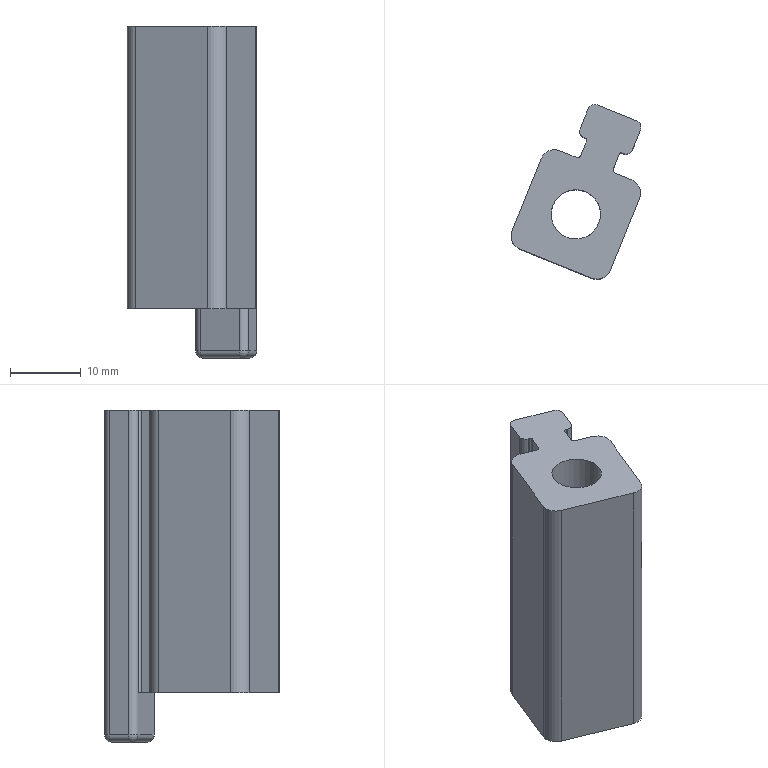Part | NX | features PS-13 2 | 1 solid | 37 faces | box 18.38 x 24.724 x 47 mm | volume 8910 mm3 | cylinder 18 | plane 15 | sphere 4 | commonest cylinder face diameters 2 x8 4 x4 0.6 x2 1 x2 7 x1 11 x1
STEP:
#1=CARTESIAN_POINT('',(2674.028,-826.139,860.716));
#2=VERTEX_POINT('',#1);
#3=CARTESIAN_POINT('',(2671.712,-825.199,860.716));
#4=VERTEX_POINT('',#3);
#5=CARTESIAN_POINT('',(89.829,221.566,860.716));
#6=DIRECTION('',(-0.9267,0.3757,0.));
#7=VECTOR('',#6,1000.);
#8=LINE('',#5,#7);
#9=EDGE_CURVE('',#2,#4,#8,.T.);
#10=ORIENTED_EDGE('',*,*,#9,.T.);
#11=CARTESIAN_POINT('',(2671.712,-825.199,900.716));
#12=VERTEX_POINT('',#11);
#13=CARTESIAN_POINT('',(2671.712,-825.199,900.716));
#14=DIRECTION('',(0.000000001,0.000000001,1.));
#15=VECTOR('',#14,1000.);
#16=LINE('',#13,#15);
#17=EDGE_CURVE('',#4,#12,#16,.T.);
#18=ORIENTED_EDGE('',*,*,#17,.T.);
#19=CARTESIAN_POINT('',(2674.028,-826.139,900.716));
#20=VERTEX_POINT('',#19);
#21=CARTESIAN_POINT('',(687.415,-20.712,900.716));
#22=DIRECTION('',(0.9267,-0.3757,0.));
#23=VECTOR('',#22,1000.);
#24=LINE('',#21,#23);
#25=EDGE_CURVE('',#20,#12,#24,.F.);
#26=ORIENTED_EDGE('',*,*,#25,.F.);
#27=CARTESIAN_POINT('',(2674.028,-826.139,880.716));
#28=DIRECTION('',(-0.000000001,-0.000000001,-1.));
#29=VECTOR('',#28,1000.);
#30=LINE('',#27,#29);
#31=EDGE_CURVE('',#20,#2,#30,.T.);
#32=ORIENTED_EDGE('',*,*,#31,.T.);
#33=EDGE_LOOP('',(#10,#18,#26,#32));
#34=FACE_BOUND('',#33,.T.);
#35=CARTESIAN_POINT('',(2672.638,-825.575,880.716));
#36=DIRECTION('',(0.3757,0.9267,-0.000000001));
#37=DIRECTION('',(-0.9267,0.3757,0.));
#38=AXIS2_PLACEMENT_3D('',#35,#36,#37);
#39=PLANE('',#38);
#40=ADVANCED_FACE('',(#34),#39,.T.);
#41=CARTESIAN_POINT('',(2666.151,-822.945,900.716));
#42=VERTEX_POINT('',#41);
#43=CARTESIAN_POINT('',(2663.834,-822.006,900.716));
#44=VERTEX_POINT('',#43);
#45=CARTESIAN_POINT('',(687.415,-20.712,900.716));
#46=DIRECTION('',(0.9267,-0.3757,0.));
#47=VECTOR('',#46,1000.);
#48=LINE('',#45,#47);
#49=EDGE_CURVE('',#42,#44,#48,.F.);
#50=ORIENTED_EDGE('',*,*,#49,.F.);
#51=CARTESIAN_POINT('',(2666.151,-822.945,860.716));
#52=VERTEX_POINT('',#51);
#53=CARTESIAN_POINT('',(2666.151,-822.945,860.716));
#54=DIRECTION('',(0.000000001,0.000000001,1.));
#55=VECTOR('',#54,1000.);
#56=LINE('',#53,#55);
#57=EDGE_CURVE('',#42,#52,#56,.F.);
#58=ORIENTED_EDGE('',*,*,#57,.T.);
#59=CARTESIAN_POINT('',(2663.834,-822.006,860.716));
#60=VERTEX_POINT('',#59);
#61=CARTESIAN_POINT('',(89.829,221.566,860.716));
#62=DIRECTION('',(-0.9267,0.3757,0.));
#63=VECTOR('',#62,1000.);
#64=LINE('',#61,#63);
#65=EDGE_CURVE('',#52,#60,#64,.T.);
#66=ORIENTED_EDGE('',*,*,#65,.T.);
#67=CARTESIAN_POINT('',(2663.834,-822.006,880.716));
#68=DIRECTION('',(-0.000000001,-0.000000001,-1.));
#69=VECTOR('',#68,1000.);
#70=LINE('',#67,#69);
#71=EDGE_CURVE('',#60,#44,#70,.F.);
#72=ORIENTED_EDGE('',*,*,#71,.T.);
#73=EDGE_LOOP('',(#50,#58,#66,#72));
#74=FACE_BOUND('',#73,.T.);
#75=CARTESIAN_POINT('',(2672.638,-825.575,880.716));
#76=DIRECTION('',(0.3757,0.9267,-0.000000001));
#77=DIRECTION('',(-0.9267,0.3757,0.));
#78=AXIS2_PLACEMENT_3D('',#75,#76,#77);
#79=PLANE('',#78);
#80=ADVANCED_FACE('',(#74),#79,.T.);
#81=CARTESIAN_POINT('',(2661.229,-823.108,860.716));
#82=VERTEX_POINT('',#81);
#83=CARTESIAN_POINT('',(2657.096,-833.302,860.716));
#84=VERTEX_POINT('',#83);
#85=CARTESIAN_POINT('',(2572.152,-1042.82,860.716));
#86=DIRECTION('',(-0.3757,-0.9267,0.000000001));
#87=VECTOR('',#86,1000.);
#88=LINE('',#85,#87);
#89=EDGE_CURVE('',#82,#84,#88,.T.);
#90=ORIENTED_EDGE('',*,*,#89,.T.);
#91=CARTESIAN_POINT('',(2657.096,-833.302,900.716));
#92=VERTEX_POINT('',#91);
#93=CARTESIAN_POINT('',(2657.096,-833.302,895.716));
#94=DIRECTION('',(0.000000001,0.000000001,1.));
#95=VECTOR('',#94,1000.);
#96=LINE('',#93,#95);
#97=EDGE_CURVE('',#84,#92,#96,.T.);
#98=ORIENTED_EDGE('',*,*,#97,.T.);
#99=CARTESIAN_POINT('',(2661.229,-823.108,900.716));
#100=VERTEX_POINT('',#99);
#101=CARTESIAN_POINT('',(1974.566,-2516.787,900.716));
#102=DIRECTION('',(-0.3757,-0.9267,0.));
#103=VECTOR('',#102,1000.);
#104=LINE('',#101,#103);
#105=EDGE_CURVE('',#100,#92,#104,.T.);
#106=ORIENTED_EDGE('',*,*,#105,.F.);
#107=CARTESIAN_POINT('',(2661.229,-823.108,895.716));
#108=DIRECTION('',(-0.000000001,-0.000000001,-1.));
#109=VECTOR('',#108,1000.);
#110=LINE('',#107,#109);
#111=EDGE_CURVE('',#100,#82,#110,.T.);
#112=ORIENTED_EDGE('',*,*,#111,.T.);
#113=EDGE_LOOP('',(#90,#98,#106,#112));
#114=FACE_BOUND('',#113,.T.);
#115=CARTESIAN_POINT('',(2663.127,-818.428,895.716));
#116=DIRECTION('',(-0.9267,0.3757,0.));
#117=DIRECTION('',(-0.3757,-0.9267,0.));
#118=AXIS2_PLACEMENT_3D('',#115,#116,#117);
#119=PLANE('',#118);
#120=ADVANCED_FACE('',(#114),#119,.T.);
#121=CARTESIAN_POINT('',(2658.198,-835.907,860.716));
#122=VERTEX_POINT('',#121);
#123=CARTESIAN_POINT('',(2668.393,-840.04,860.716));
#124=VERTEX_POINT('',#123);
#125=CARTESIAN_POINT('',(84.193,207.665,860.716));
#126=DIRECTION('',(0.9267,-0.3757,0.));
#127=VECTOR('',#126,1000.);
#128=LINE('',#125,#127);
#129=EDGE_CURVE('',#122,#124,#128,.T.);
#130=ORIENTED_EDGE('',*,*,#129,.T.);
#131=CARTESIAN_POINT('',(2668.393,-840.04,900.716));
#132=VERTEX_POINT('',#131);
#133=CARTESIAN_POINT('',(2668.393,-840.04,895.716));
#134=DIRECTION('',(0.000000001,0.000000001,1.));
#135=VECTOR('',#134,1000.);
#136=LINE('',#133,#135);
#137=EDGE_CURVE('',#124,#132,#136,.T.);
#138=ORIENTED_EDGE('',*,*,#137,.T.);
#139=CARTESIAN_POINT('',(2658.198,-835.907,900.716));
#140=VERTEX_POINT('',#139);
#141=CARTESIAN_POINT('',(681.779,-34.613,900.716));
#142=DIRECTION('',(0.9267,-0.3757,0.));
#143=VECTOR('',#142,1000.);
#144=LINE('',#141,#143);
#145=EDGE_CURVE('',#140,#132,#144,.T.);
#146=ORIENTED_EDGE('',*,*,#145,.F.);
#147=CARTESIAN_POINT('',(2658.198,-835.907,895.716));
#148=DIRECTION('',(0.000000001,0.000000001,1.));
#149=VECTOR('',#148,1000.);
#150=LINE('',#147,#149);
#151=EDGE_CURVE('',#140,#122,#150,.F.);
#152=ORIENTED_EDGE('',*,*,#151,.T.);
#153=EDGE_LOOP('',(#130,#138,#146,#152));
#154=FACE_BOUND('',#153,.T.);
#155=CARTESIAN_POINT('',(2660.527,-836.85,895.716));
#156=DIRECTION('',(-0.3757,-0.9267,0.000000001));
#157=DIRECTION('',(0.9267,-0.3757,0.));
#158=AXIS2_PLACEMENT_3D('',#155,#156,#157);
#159=PLANE('',#158);
#160=ADVANCED_FACE('',(#154),#159,.T.);
#161=CARTESIAN_POINT('',(2670.997,-838.938,900.716));
#162=VERTEX_POINT('',#161);
#163=CARTESIAN_POINT('',(2675.13,-828.743,900.716));
#164=VERTEX_POINT('',#163);
#165=CARTESIAN_POINT('',(1988.467,-2522.423,900.716));
#166=DIRECTION('',(0.3757,0.9267,0.));
#167=VECTOR('',#166,1000.);
#168=LINE('',#165,#167);
#169=EDGE_CURVE('',#162,#164,#168,.T.);
#170=ORIENTED_EDGE('',*,*,#169,.F.);
#171=CARTESIAN_POINT('',(2670.997,-838.938,860.716));
#172=VERTEX_POINT('',#171);
#173=CARTESIAN_POINT('',(2670.997,-838.938,895.716));
#174=DIRECTION('',(0.000000001,0.000000001,1.));
#175=VECTOR('',#174,1000.);
#176=LINE('',#173,#175);
#177=EDGE_CURVE('',#162,#172,#176,.F.);
#178=ORIENTED_EDGE('',*,*,#177,.T.);
#179=CARTESIAN_POINT('',(2675.13,-828.743,860.716));
#180=VERTEX_POINT('',#179);
#181=CARTESIAN_POINT('',(2586.053,-1048.456,860.716));
#182=DIRECTION('',(0.3757,0.9267,-0.000000001));
#183=VECTOR('',#182,1000.);
#184=LINE('',#181,#183);
#185=EDGE_CURVE('',#172,#180,#184,.T.);
#186=ORIENTED_EDGE('',*,*,#185,.T.);
#187=CARTESIAN_POINT('',(2675.13,-828.743,895.716));
#188=DIRECTION('',(-0.000000001,-0.000000001,-1.));
#189=VECTOR('',#188,1000.);
#190=LINE('',#187,#189);
#191=EDGE_CURVE('',#180,#164,#190,.F.);
#192=ORIENTED_EDGE('',*,*,#191,.T.);
#193=EDGE_LOOP('',(#170,#178,#186,#192));
#194=FACE_BOUND('',#193,.T.);
#195=CARTESIAN_POINT('',(2676.633,-825.037,895.716));
#196=DIRECTION('',(0.9267,-0.3757,0.));
#197=DIRECTION('',(0.3757,0.9267,0.));
#198=AXIS2_PLACEMENT_3D('',#195,#196,#197);
#199=PLANE('',#198);
#200=ADVANCED_FACE('',(#194),#199,.T.);
#201=CARTESIAN_POINT('',(2666.113,-836.523,860.716));
#202=VERTEX_POINT('',#201);
#203=CARTESIAN_POINT('',(2666.113,-831.023,860.716));
#204=DIRECTION('',(0.000000001,0.000000001,1.));
#205=DIRECTION('',(0.,-1.,0.000000001));
#206=AXIS2_PLACEMENT_3D('',#203,#204,#205);
#207=CIRCLE('',#206,5.5);
#208=EDGE_CURVE('',#202,#202,#207,.T.);
#209=ORIENTED_EDGE('',*,*,#208,.T.);
#210=EDGE_LOOP('',(#209));
#211=FACE_BOUND('',#210,.T.);
#212=ORIENTED_EDGE('',*,*,#185,.F.);
#213=CARTESIAN_POINT('',(2669.144,-838.186,860.716));
#214=DIRECTION('',(0.000000001,0.000000001,1.));
#215=DIRECTION('',(0.,-1.,0.000000001));
#216=AXIS2_PLACEMENT_3D('',#213,#214,#215);
#217=CIRCLE('',#216,2.);
#218=EDGE_CURVE('',#172,#124,#217,.F.);
#219=ORIENTED_EDGE('',*,*,#218,.T.);
#220=ORIENTED_EDGE('',*,*,#129,.F.);
#221=CARTESIAN_POINT('',(2658.95,-834.053,860.716));
#222=DIRECTION('',(0.000000001,0.000000001,1.));
#223=DIRECTION('',(0.,-1.,0.000000001));
#224=AXIS2_PLACEMENT_3D('',#221,#222,#223);
#225=CIRCLE('',#224,2.);
#226=EDGE_CURVE('',#122,#84,#225,.F.);
#227=ORIENTED_EDGE('',*,*,#226,.T.);
#228=ORIENTED_EDGE('',*,*,#89,.F.);
#229=CARTESIAN_POINT('',(2663.083,-823.859,860.716));
#230=DIRECTION('',(0.000000001,0.000000001,1.));
#231=DIRECTION('',(0.,-1.,0.000000001));
#232=AXIS2_PLACEMENT_3D('',#229,#230,#231);
#233=CIRCLE('',#232,2.);
#234=EDGE_CURVE('',#82,#60,#233,.F.);
#235=ORIENTED_EDGE('',*,*,#234,.T.);
#236=ORIENTED_EDGE('',*,*,#65,.F.);
#237=CARTESIAN_POINT('',(2666.802,-822.669,860.716));
#238=VERTEX_POINT('',#237);
#239=CARTESIAN_POINT('',(2666.339,-822.482,860.716));
#240=DIRECTION('',(0.000000001,0.000000001,1.));
#241=DIRECTION('',(0.,-1.,0.000000001));
#242=AXIS2_PLACEMENT_3D('',#239,#240,#241);
#243=CIRCLE('',#242,0.5);
#244=EDGE_CURVE('',#52,#238,#243,.T.);
#245=ORIENTED_EDGE('',*,*,#244,.T.);
#246=CARTESIAN_POINT('',(2667.629,-820.631,860.716));
#247=VERTEX_POINT('',#246);
#248=CARTESIAN_POINT('',(2576.786,-1044.699,860.716));
#249=DIRECTION('',(-0.3757,-0.9267,0.000000001));
#250=VECTOR('',#249,1000.);
#251=LINE('',#248,#250);
#252=EDGE_CURVE('',#247,#238,#251,.T.);
#253=ORIENTED_EDGE('',*,*,#252,.F.);
#254=CARTESIAN_POINT('',(2667.464,-820.24,860.716));
#255=VERTEX_POINT('',#254);
#256=CARTESIAN_POINT('',(2667.351,-820.518,860.716));
#257=DIRECTION('',(0.000000001,0.000000001,1.));
#258=DIRECTION('',(0.,-1.,0.000000001));
#259=AXIS2_PLACEMENT_3D('',#256,#257,#258);
#260=CIRCLE('',#259,0.3);
#261=EDGE_CURVE('',#247,#255,#260,.T.);
#262=ORIENTED_EDGE('',*,*,#261,.T.);
#263=CARTESIAN_POINT('',(2672.653,-822.344,860.716));
#264=VERTEX_POINT('',#263);
#265=CARTESIAN_POINT('',(2670.058,-821.292,860.716));
#266=DIRECTION('',(0.9267,-0.3757,0.));
#267=VECTOR('',#266,1000.);
#268=LINE('',#265,#267);
#269=EDGE_CURVE('',#255,#264,#268,.T.);
#270=ORIENTED_EDGE('',*,*,#269,.T.);
#271=CARTESIAN_POINT('',(2672.263,-822.509,860.716));
#272=VERTEX_POINT('',#271);
#273=CARTESIAN_POINT('',(2672.541,-822.622,860.716));
#274=DIRECTION('',(0.000000001,0.000000001,1.));
#275=DIRECTION('',(0.,-1.,0.000000001));
#276=AXIS2_PLACEMENT_3D('',#273,#274,#275);
#277=CIRCLE('',#276,0.3);
#278=EDGE_CURVE('',#264,#272,#277,.T.);
#279=ORIENTED_EDGE('',*,*,#278,.T.);
#280=CARTESIAN_POINT('',(2671.436,-824.548,860.716));
#281=VERTEX_POINT('',#280);
#282=CARTESIAN_POINT('',(2581.419,-1046.577,860.716));
#283=DIRECTION('',(0.3757,0.9267,-0.000000001));
#284=VECTOR('',#283,1000.);
#285=LINE('',#282,#284);
#286=EDGE_CURVE('',#281,#272,#285,.T.);
#287=ORIENTED_EDGE('',*,*,#286,.F.);
#288=CARTESIAN_POINT('',(2671.899,-824.736,860.716));
#289=DIRECTION('',(0.000000001,0.000000001,1.));
#290=DIRECTION('',(0.,-1.,0.000000001));
#291=AXIS2_PLACEMENT_3D('',#288,#289,#290);
#292=CIRCLE('',#291,0.5);
#293=EDGE_CURVE('',#281,#4,#292,.T.);
#294=ORIENTED_EDGE('',*,*,#293,.T.);
#295=ORIENTED_EDGE('',*,*,#9,.F.);
#296=CARTESIAN_POINT('',(2673.277,-827.992,860.716));
#297=DIRECTION('',(0.000000001,0.000000001,1.));
#298=DIRECTION('',(0.,-1.,0.000000001));
#299=AXIS2_PLACEMENT_3D('',#296,#297,#298);
#300=CIRCLE('',#299,2.);
#301=EDGE_CURVE('',#2,#180,#300,.F.);
#302=ORIENTED_EDGE('',*,*,#301,.T.);
#303=EDGE_LOOP('',(#212,#219,#220,#227,#228,#235,#236,#245,#253,#262,#270,#279,#287,#294,#295,#302));
#304=FACE_BOUND('',#303,.T.);
#305=CARTESIAN_POINT('',(0.000000481,0.000001186,860.716));
#306=DIRECTION('',(0.000000001,0.000000001,1.));
#307=DIRECTION('',(0.,-1.,0.000000001));
#308=AXIS2_PLACEMENT_3D('',#305,#306,#307);
#309=PLANE('',#308);
#310=ADVANCED_FACE('',(#211,#304),#309,.F.);
#311=CARTESIAN_POINT('',(2669.613,-831.023,900.716));
#312=VERTEX_POINT('',#311);
#313=CARTESIAN_POINT('',(2666.113,-831.023,900.716));
#314=DIRECTION('',(0.,0.,1.));
#315=DIRECTION('',(1.,0.,0.));
#316=AXIS2_PLACEMENT_3D('',#313,#314,#315);
#317=CIRCLE('',#316,3.5);
#318=EDGE_CURVE('',#312,#312,#317,.T.);
#319=ORIENTED_EDGE('',*,*,#318,.F.);
#320=EDGE_LOOP('',(#319));
#321=FACE_BOUND('',#320,.T.);
#322=ORIENTED_EDGE('',*,*,#145,.T.);
#323=CARTESIAN_POINT('',(2669.144,-838.186,900.716));
#324=DIRECTION('',(0.,0.,1.));
#325=DIRECTION('',(1.,0.,0.));
#326=AXIS2_PLACEMENT_3D('',#323,#324,#325);
#327=CIRCLE('',#326,2.);
#328=EDGE_CURVE('',#132,#162,#327,.T.);
#329=ORIENTED_EDGE('',*,*,#328,.T.);
#330=ORIENTED_EDGE('',*,*,#169,.T.);
#331=CARTESIAN_POINT('',(2673.277,-827.992,900.716));
#332=DIRECTION('',(0.,0.,1.));
#333=DIRECTION('',(1.,0.,0.));
#334=AXIS2_PLACEMENT_3D('',#331,#332,#333);
#335=CIRCLE('',#334,2.);
#336=EDGE_CURVE('',#164,#20,#335,.T.);
#337=ORIENTED_EDGE('',*,*,#336,.T.);
#338=ORIENTED_EDGE('',*,*,#25,.T.);
#339=CARTESIAN_POINT('',(2671.436,-824.548,900.716));
#340=VERTEX_POINT('',#339);
#341=CARTESIAN_POINT('',(2671.899,-824.736,900.716));
#342=DIRECTION('',(0.,0.,1.));
#343=DIRECTION('',(1.,0.,0.));
#344=AXIS2_PLACEMENT_3D('',#341,#342,#343);
#345=CIRCLE('',#344,0.5);
#346=EDGE_CURVE('',#12,#340,#345,.F.);
#347=ORIENTED_EDGE('',*,*,#346,.T.);
#348=CARTESIAN_POINT('',(2672.263,-822.509,900.716));
#349=VERTEX_POINT('',#348);
#350=CARTESIAN_POINT('',(2581.419,-1046.577,900.716));
#351=DIRECTION('',(0.3757,0.9267,-0.000000001));
#352=VECTOR('',#351,1000.);
#353=LINE('',#350,#352);
#354=EDGE_CURVE('',#340,#349,#353,.T.);
#355=ORIENTED_EDGE('',*,*,#354,.T.);
#356=CARTESIAN_POINT('',(2672.653,-822.344,900.716));
#357=VERTEX_POINT('',#356);
#358=CARTESIAN_POINT('',(2672.541,-822.622,900.716));
#359=DIRECTION('',(0.,0.,1.));
#360=DIRECTION('',(1.,0.,0.));
#361=AXIS2_PLACEMENT_3D('',#358,#359,#360);
#362=CIRCLE('',#361,0.3);
#363=EDGE_CURVE('',#349,#357,#362,.F.);
#364=ORIENTED_EDGE('',*,*,#363,.T.);
#365=CARTESIAN_POINT('',(2672.827,-822.414,900.716));
#366=VERTEX_POINT('',#365);
#367=CARTESIAN_POINT('',(2670.058,-821.292,900.716));
#368=DIRECTION('',(-0.9267,0.3757,0.));
#369=VECTOR('',#368,1000.);
#370=LINE('',#367,#369);
#371=EDGE_CURVE('',#366,#357,#370,.T.);
#372=ORIENTED_EDGE('',*,*,#371,.F.);
#373=CARTESIAN_POINT('',(2674.13,-821.863,900.716));
#374=VERTEX_POINT('',#373);
#375=CARTESIAN_POINT('',(2673.203,-821.488,900.716));
#376=DIRECTION('',(0.,0.,-1.));
#377=DIRECTION('',(1.,0.,0.));
#378=AXIS2_PLACEMENT_3D('',#375,#376,#377);
#379=CIRCLE('',#378,1.);
#380=EDGE_CURVE('',#374,#366,#379,.T.);
#381=ORIENTED_EDGE('',*,*,#380,.F.);
#382=CARTESIAN_POINT('',(2675.257,-819.083,900.716));
#383=VERTEX_POINT('',#382);
#384=CARTESIAN_POINT('',(2676.384,-816.303,900.716));
#385=DIRECTION('',(-0.3757,-0.9267,0.));
#386=VECTOR('',#385,1000.);
#387=LINE('',#384,#386);
#388=EDGE_CURVE('',#374,#383,#387,.F.);
#389=ORIENTED_EDGE('',*,*,#388,.T.);
#390=CARTESIAN_POINT('',(2674.706,-817.781,900.716));
#391=VERTEX_POINT('',#390);
#392=CARTESIAN_POINT('',(2674.33,-818.708,900.716));
#393=DIRECTION('',(0.,0.,-1.));
#394=DIRECTION('',(1.,0.,0.));
#395=AXIS2_PLACEMENT_3D('',#392,#393,#394);
#396=CIRCLE('',#395,1.);
#397=EDGE_CURVE('',#391,#383,#396,.T.);
#398=ORIENTED_EDGE('',*,*,#397,.F.);
#399=CARTESIAN_POINT('',(2669.168,-815.536,900.716));
#400=VERTEX_POINT('',#399);
#401=CARTESIAN_POINT('',(2671.937,-816.658,900.716));
#402=DIRECTION('',(-0.9267,0.3757,0.));
#403=VECTOR('',#402,1000.);
#404=LINE('',#401,#403);
#405=EDGE_CURVE('',#391,#400,#404,.T.);
#406=ORIENTED_EDGE('',*,*,#405,.T.);
#407=CARTESIAN_POINT('',(2667.866,-816.087,900.716));
#408=VERTEX_POINT('',#407);
#409=CARTESIAN_POINT('',(2668.792,-816.462,900.716));
#410=DIRECTION('',(0.,0.,-1.));
#411=DIRECTION('',(1.,0.,0.));
#412=AXIS2_PLACEMENT_3D('',#409,#410,#411);
#413=CIRCLE('',#412,1.);
#414=EDGE_CURVE('',#408,#400,#413,.T.);
#415=ORIENTED_EDGE('',*,*,#414,.F.);
#416=CARTESIAN_POINT('',(2666.739,-818.867,900.716));
#417=VERTEX_POINT('',#416);
#418=CARTESIAN_POINT('',(2668.993,-813.306,900.716));
#419=DIRECTION('',(-0.3757,-0.9267,0.));
#420=VECTOR('',#419,1000.);
#421=LINE('',#418,#420);
#422=EDGE_CURVE('',#408,#417,#421,.T.);
#423=ORIENTED_EDGE('',*,*,#422,.T.);
#424=CARTESIAN_POINT('',(2667.29,-820.169,900.716));
#425=VERTEX_POINT('',#424);
#426=CARTESIAN_POINT('',(2667.665,-819.243,900.716));
#427=DIRECTION('',(0.,0.,-1.));
#428=DIRECTION('',(1.,0.,0.));
#429=AXIS2_PLACEMENT_3D('',#426,#427,#428);
#430=CIRCLE('',#429,1.);
#431=EDGE_CURVE('',#425,#417,#430,.T.);
#432=ORIENTED_EDGE('',*,*,#431,.F.);
#433=CARTESIAN_POINT('',(2667.464,-820.24,900.716));
#434=VERTEX_POINT('',#433);
#435=CARTESIAN_POINT('',(2670.058,-821.292,900.716));
#436=DIRECTION('',(-0.9267,0.3757,0.));
#437=VECTOR('',#436,1000.);
#438=LINE('',#435,#437);
#439=EDGE_CURVE('',#434,#425,#438,.T.);
#440=ORIENTED_EDGE('',*,*,#439,.F.);
#441=CARTESIAN_POINT('',(2667.629,-820.631,900.716));
#442=VERTEX_POINT('',#441);
#443=CARTESIAN_POINT('',(2667.351,-820.518,900.716));
#444=DIRECTION('',(0.,0.,1.));
#445=DIRECTION('',(1.,0.,0.));
#446=AXIS2_PLACEMENT_3D('',#443,#444,#445);
#447=CIRCLE('',#446,0.3);
#448=EDGE_CURVE('',#434,#442,#447,.F.);
#449=ORIENTED_EDGE('',*,*,#448,.T.);
#450=CARTESIAN_POINT('',(2666.802,-822.669,900.716));
#451=VERTEX_POINT('',#450);
#452=CARTESIAN_POINT('',(2576.786,-1044.699,900.716));
#453=DIRECTION('',(-0.3757,-0.9267,0.000000001));
#454=VECTOR('',#453,1000.);
#455=LINE('',#452,#454);
#456=EDGE_CURVE('',#442,#451,#455,.T.);
#457=ORIENTED_EDGE('',*,*,#456,.T.);
#458=CARTESIAN_POINT('',(2666.339,-822.482,900.716));
#459=DIRECTION('',(0.,0.,1.));
#460=DIRECTION('',(1.,0.,0.));
#461=AXIS2_PLACEMENT_3D('',#458,#459,#460);
#462=CIRCLE('',#461,0.5);
#463=EDGE_CURVE('',#451,#42,#462,.F.);
#464=ORIENTED_EDGE('',*,*,#463,.T.);
#465=ORIENTED_EDGE('',*,*,#49,.T.);
#466=CARTESIAN_POINT('',(2663.083,-823.859,900.716));
#467=DIRECTION('',(0.,0.,1.));
#468=DIRECTION('',(1.,0.,0.));
#469=AXIS2_PLACEMENT_3D('',#466,#467,#468);
#470=CIRCLE('',#469,2.);
#471=EDGE_CURVE('',#44,#100,#470,.T.);
#472=ORIENTED_EDGE('',*,*,#471,.T.);
#473=ORIENTED_EDGE('',*,*,#105,.T.);
#474=CARTESIAN_POINT('',(2658.95,-834.053,900.716));
#475=DIRECTION('',(0.,0.,1.));
#476=DIRECTION('',(1.,0.,0.));
#477=AXIS2_PLACEMENT_3D('',#474,#475,#476);
#478=CIRCLE('',#477,2.);
#479=EDGE_CURVE('',#92,#140,#478,.T.);
#480=ORIENTED_EDGE('',*,*,#479,.T.);
#481=EDGE_LOOP('',(#322,#329,#330,#337,#338,#347,#355,#364,#372,#381,#389,#398,#406,#415,#423,#432,#440,#449,#457,#464,#465,#472,#473,#480));
#482=FACE_BOUND('',#481,.T.);
#483=CARTESIAN_POINT('',(0.,-1716.245,900.716));
#484=DIRECTION('',(0.,0.,1.));
#485=DIRECTION('',(1.,0.,0.));
#486=AXIS2_PLACEMENT_3D('',#483,#484,#485);
#487=PLANE('',#486);
#488=ADVANCED_FACE('',(#321,#482),#487,.T.);
#489=ORIENTED_EDGE('',*,*,#218,.F.);
#490=ORIENTED_EDGE('',*,*,#177,.F.);
#491=ORIENTED_EDGE('',*,*,#328,.F.);
#492=ORIENTED_EDGE('',*,*,#137,.F.);
#493=EDGE_LOOP('',(#489,#490,#491,#492));
#494=FACE_BOUND('',#493,.T.);
#495=CARTESIAN_POINT('',(2669.144,-838.186,895.716));
#496=DIRECTION('',(0.000000001,0.000000001,1.));
#497=DIRECTION('',(0.,-1.,0.000000001));
#498=AXIS2_PLACEMENT_3D('',#495,#496,#497);
#499=CYLINDRICAL_SURFACE('',#498,2.);
#500=ADVANCED_FACE('',(#494),#499,.T.);
#501=ORIENTED_EDGE('',*,*,#336,.F.);
#502=ORIENTED_EDGE('',*,*,#191,.F.);
#503=ORIENTED_EDGE('',*,*,#301,.F.);
#504=ORIENTED_EDGE('',*,*,#31,.F.);
#505=EDGE_LOOP('',(#501,#502,#503,#504));
#506=FACE_BOUND('',#505,.T.);
#507=CARTESIAN_POINT('',(2673.277,-827.992,880.716));
#508=DIRECTION('',(-0.000000001,-0.000000001,-1.));
#509=DIRECTION('',(0.,1.,-0.000000001));
#510=AXIS2_PLACEMENT_3D('',#507,#508,#509);
#511=CYLINDRICAL_SURFACE('',#510,2.);
#512=ADVANCED_FACE('',(#506),#511,.T.);
#513=ORIENTED_EDGE('',*,*,#226,.F.);
#514=ORIENTED_EDGE('',*,*,#151,.F.);
#515=ORIENTED_EDGE('',*,*,#479,.F.);
#516=ORIENTED_EDGE('',*,*,#97,.F.);
#517=EDGE_LOOP('',(#513,#514,#515,#516));
#518=FACE_BOUND('',#517,.T.);
#519=CARTESIAN_POINT('',(2658.95,-834.053,895.716));
#520=DIRECTION('',(0.000000001,0.000000001,1.));
#521=DIRECTION('',(0.,-1.,0.000000001));
#522=AXIS2_PLACEMENT_3D('',#519,#520,#521);
#523=CYLINDRICAL_SURFACE('',#522,2.);
#524=ADVANCED_FACE('',(#518),#523,.T.);
#525=ORIENTED_EDGE('',*,*,#471,.F.);
#526=ORIENTED_EDGE('',*,*,#71,.F.);
#527=ORIENTED_EDGE('',*,*,#234,.F.);
#528=ORIENTED_EDGE('',*,*,#111,.F.);
#529=EDGE_LOOP('',(#525,#526,#527,#528));
#530=FACE_BOUND('',#529,.T.);
#531=CARTESIAN_POINT('',(2663.083,-823.859,895.716));
#532=DIRECTION('',(-0.000000001,-0.000000001,-1.));
#533=DIRECTION('',(0.,1.,-0.000000001));
#534=AXIS2_PLACEMENT_3D('',#531,#532,#533);
#535=CYLINDRICAL_SURFACE('',#534,2.);
#536=ADVANCED_FACE('',(#530),#535,.T.);
#537=CARTESIAN_POINT('',(2668.18,-825.926,875.716));
#538=VERTEX_POINT('',#537);
#539=CARTESIAN_POINT('',(2666.113,-831.023,875.716));
#540=DIRECTION('',(-0.000000001,-0.000000001,-1.));
#541=DIRECTION('',(0.3757,0.9267,-0.000000001));
#542=AXIS2_PLACEMENT_3D('',#539,#540,#541);
#543=CIRCLE('',#542,5.5);
#544=EDGE_CURVE('',#538,#538,#543,.F.);
#545=ORIENTED_EDGE('',*,*,#544,.T.);
#546=EDGE_LOOP('',(#545));
#547=FACE_BOUND('',#546,.T.);
#548=ORIENTED_EDGE('',*,*,#208,.F.);
#549=EDGE_LOOP('',(#548));
#550=FACE_BOUND('',#549,.T.);
#551=CARTESIAN_POINT('',(2666.113,-831.023,875.716));
#552=DIRECTION('',(-0.000000001,-0.000000001,-1.));
#553=DIRECTION('',(0.,1.,-0.000000001));
#554=AXIS2_PLACEMENT_3D('',#551,#552,#553);
#555=CYLINDRICAL_SURFACE('',#554,5.5);
#556=ADVANCED_FACE('',(#547,#550),#555,.F.);
#557=ORIENTED_EDGE('',*,*,#318,.T.);
#558=EDGE_LOOP('',(#557));
#559=FACE_BOUND('',#558,.T.);
#560=CARTESIAN_POINT('',(2666.113,-827.523,875.716));
#561=VERTEX_POINT('',#560);
#562=CARTESIAN_POINT('',(2666.113,-831.023,875.716));
#563=DIRECTION('',(-0.000000001,-0.000000001,-1.));
#564=DIRECTION('',(0.,1.,-0.000000001));
#565=AXIS2_PLACEMENT_3D('',#562,#563,#564);
#566=CIRCLE('',#565,3.5);
#567=EDGE_CURVE('',#561,#561,#566,.T.);
#568=ORIENTED_EDGE('',*,*,#567,.T.);
#569=EDGE_LOOP('',(#568));
#570=FACE_BOUND('',#569,.T.);
#571=CARTESIAN_POINT('',(2666.113,-831.023,901.716));
#572=DIRECTION('',(-0.000000001,-0.000000001,-1.));
#573=DIRECTION('',(0.,1.,-0.000000001));
#574=AXIS2_PLACEMENT_3D('',#571,#572,#573);
#575=CYLINDRICAL_SURFACE('',#574,3.5);
#576=ADVANCED_FACE('',(#559,#570),#575,.F.);
#577=ORIENTED_EDGE('',*,*,#567,.F.);
#578=EDGE_LOOP('',(#577));
#579=FACE_BOUND('',#578,.T.);
#580=ORIENTED_EDGE('',*,*,#544,.F.);
#581=EDGE_LOOP('',(#580));
#582=FACE_BOUND('',#581,.T.);
#583=CARTESIAN_POINT('',(2666.113,-831.023,875.716));
#584=DIRECTION('',(-0.000000001,-0.000000001,-1.));
#585=DIRECTION('',(0.,1.,-0.000000001));
#586=AXIS2_PLACEMENT_3D('',#583,#584,#585);
#587=PLANE('',#586);
#588=ADVANCED_FACE('',(#579,#582),#587,.T.);
#589=ORIENTED_EDGE('',*,*,#354,.F.);
#590=CARTESIAN_POINT('',(2671.436,-824.548,860.716));
#591=DIRECTION('',(0.000000001,0.000000001,1.));
#592=VECTOR('',#591,1000.);
#593=LINE('',#590,#592);
#594=EDGE_CURVE('',#340,#281,#593,.F.);
#595=ORIENTED_EDGE('',*,*,#594,.T.);
#596=ORIENTED_EDGE('',*,*,#286,.T.);
#597=CARTESIAN_POINT('',(2672.263,-822.509,895.716));
#598=DIRECTION('',(-0.000000001,-0.000000001,-1.));
#599=VECTOR('',#598,1000.);
#600=LINE('',#597,#599);
#601=EDGE_CURVE('',#272,#349,#600,.F.);
#602=ORIENTED_EDGE('',*,*,#601,.T.);
#603=EDGE_LOOP('',(#589,#595,#596,#602));
#604=FACE_BOUND('',#603,.T.);
#605=CARTESIAN_POINT('',(2672.,-823.158,895.716));
#606=DIRECTION('',(0.9267,-0.3757,0.));
#607=DIRECTION('',(0.3757,0.9267,0.));
#608=AXIS2_PLACEMENT_3D('',#605,#606,#607);
#609=PLANE('',#608);
#610=ADVANCED_FACE('',(#604),#609,.T.);
#611=ORIENTED_EDGE('',*,*,#252,.T.);
#612=CARTESIAN_POINT('',(2666.802,-822.669,900.716));
#613=DIRECTION('',(0.000000001,0.000000001,1.));
#614=VECTOR('',#613,1000.);
#615=LINE('',#612,#614);
#616=EDGE_CURVE('',#238,#451,#615,.T.);
#617=ORIENTED_EDGE('',*,*,#616,.T.);
#618=ORIENTED_EDGE('',*,*,#456,.F.);
#619=CARTESIAN_POINT('',(2667.629,-820.631,895.716));
#620=DIRECTION('',(0.000000001,0.000000001,1.));
#621=VECTOR('',#620,1000.);
#622=LINE('',#619,#621);
#623=EDGE_CURVE('',#442,#247,#622,.F.);
#624=ORIENTED_EDGE('',*,*,#623,.T.);
#625=EDGE_LOOP('',(#611,#617,#618,#624));
#626=FACE_BOUND('',#625,.T.);
#627=CARTESIAN_POINT('',(2667.76,-820.306,895.716));
#628=DIRECTION('',(-0.9267,0.3757,0.));
#629=DIRECTION('',(-0.3757,-0.9267,0.));
#630=AXIS2_PLACEMENT_3D('',#627,#628,#629);
#631=PLANE('',#630);
#632=ADVANCED_FACE('',(#626),#631,.T.);
#633=CARTESIAN_POINT('',(2669.168,-815.536,854.716));
#634=VERTEX_POINT('',#633);
#635=CARTESIAN_POINT('',(2669.168,-815.536,857.716));
#636=DIRECTION('',(0.000000008,-0.000000001,1.));
#637=VECTOR('',#636,1000.);
#638=LINE('',#635,#637);
#639=EDGE_CURVE('',#400,#634,#638,.F.);
#640=ORIENTED_EDGE('',*,*,#639,.F.);
#641=ORIENTED_EDGE('',*,*,#405,.F.);
#642=CARTESIAN_POINT('',(2674.706,-817.781,854.716));
#643=VERTEX_POINT('',#642);
#644=CARTESIAN_POINT('',(2674.706,-817.781,857.716));
#645=DIRECTION('',(-0.000000008,0.000000001,-1.));
#646=VECTOR('',#645,1000.);
#647=LINE('',#644,#646);
#648=EDGE_CURVE('',#643,#391,#647,.F.);
#649=ORIENTED_EDGE('',*,*,#648,.F.);
#650=CARTESIAN_POINT('',(2671.937,-816.658,854.716));
#651=DIRECTION('',(0.9267,-0.3757,0.));
#652=VECTOR('',#651,1000.);
#653=LINE('',#650,#652);
#654=EDGE_CURVE('',#634,#643,#653,.T.);
#655=ORIENTED_EDGE('',*,*,#654,.F.);
#656=EDGE_LOOP('',(#640,#641,#649,#655));
#657=FACE_BOUND('',#656,.T.);
#658=CARTESIAN_POINT('',(2671.937,-816.658,857.716));
#659=DIRECTION('',(0.3757,0.9267,-0.000000001));
#660=DIRECTION('',(0.9267,-0.3757,0.));
#661=AXIS2_PLACEMENT_3D('',#658,#659,#660);
#662=PLANE('',#661);
#663=ADVANCED_FACE('',(#657),#662,.T.);
#664=CARTESIAN_POINT('',(2666.739,-818.867,854.716));
#665=VERTEX_POINT('',#664);
#666=CARTESIAN_POINT('',(2666.739,-818.867,857.716));
#667=DIRECTION('',(-0.000000008,0.000000001,-1.));
#668=VECTOR('',#667,1000.);
#669=LINE('',#666,#668);
#670=EDGE_CURVE('',#417,#665,#669,.T.);
#671=ORIENTED_EDGE('',*,*,#670,.F.);
#672=ORIENTED_EDGE('',*,*,#422,.F.);
#673=CARTESIAN_POINT('',(2667.866,-816.087,854.716));
#674=VERTEX_POINT('',#673);
#675=CARTESIAN_POINT('',(2667.866,-816.087,857.716));
#676=DIRECTION('',(0.000000008,-0.000000001,1.));
#677=VECTOR('',#676,1000.);
#678=LINE('',#675,#677);
#679=EDGE_CURVE('',#674,#408,#678,.T.);
#680=ORIENTED_EDGE('',*,*,#679,.F.);
#681=CARTESIAN_POINT('',(2668.993,-813.306,854.716));
#682=DIRECTION('',(0.3757,0.9267,0.));
#683=VECTOR('',#682,1000.);
#684=LINE('',#681,#683);
#685=EDGE_CURVE('',#665,#674,#684,.T.);
#686=ORIENTED_EDGE('',*,*,#685,.F.);
#687=EDGE_LOOP('',(#671,#672,#680,#686));
#688=FACE_BOUND('',#687,.T.);
#689=CARTESIAN_POINT('',(2668.993,-813.306,857.716));
#690=DIRECTION('',(-0.9267,0.3757,0.000000008));
#691=DIRECTION('',(0.3757,0.9267,0.));
#692=AXIS2_PLACEMENT_3D('',#689,#690,#691);
#693=PLANE('',#692);
#694=ADVANCED_FACE('',(#688),#693,.T.);
#695=CARTESIAN_POINT('',(2675.257,-819.083,854.716));
#696=VERTEX_POINT('',#695);
#697=CARTESIAN_POINT('',(2675.257,-819.083,857.716));
#698=DIRECTION('',(0.000000008,-0.000000001,1.));
#699=VECTOR('',#698,1000.);
#700=LINE('',#697,#699);
#701=EDGE_CURVE('',#383,#696,#700,.F.);
#702=ORIENTED_EDGE('',*,*,#701,.F.);
#703=ORIENTED_EDGE('',*,*,#388,.F.);
#704=CARTESIAN_POINT('',(2674.13,-821.863,854.716));
#705=VERTEX_POINT('',#704);
#706=CARTESIAN_POINT('',(2674.13,-821.863,901.716));
#707=DIRECTION('',(-0.000000008,0.000000001,-1.));
#708=VECTOR('',#707,1000.);
#709=LINE('',#706,#708);
#710=EDGE_CURVE('',#705,#374,#709,.F.);
#711=ORIENTED_EDGE('',*,*,#710,.F.);
#712=CARTESIAN_POINT('',(2676.384,-816.303,854.716));
#713=DIRECTION('',(-0.3757,-0.9267,0.));
#714=VECTOR('',#713,1000.);
#715=LINE('',#712,#714);
#716=EDGE_CURVE('',#696,#705,#715,.T.);
#717=ORIENTED_EDGE('',*,*,#716,.F.);
#718=EDGE_LOOP('',(#702,#703,#711,#717));
#719=FACE_BOUND('',#718,.T.);
#720=CARTESIAN_POINT('',(2676.384,-816.303,857.716));
#721=DIRECTION('',(-0.9267,0.3757,0.000000008));
#722=DIRECTION('',(0.3757,0.9267,0.));
#723=AXIS2_PLACEMENT_3D('',#720,#721,#722);
#724=PLANE('',#723);
#725=ADVANCED_FACE('',(#719),#724,.F.);
#726=ORIENTED_EDGE('',*,*,#371,.T.);
#727=CARTESIAN_POINT('',(2672.653,-822.344,859.716));
#728=DIRECTION('',(-0.000000001,-0.000000001,-1.));
#729=VECTOR('',#728,1000.);
#730=LINE('',#727,#729);
#731=EDGE_CURVE('',#357,#264,#730,.T.);
#732=ORIENTED_EDGE('',*,*,#731,.T.);
#733=ORIENTED_EDGE('',*,*,#269,.F.);
#734=CARTESIAN_POINT('',(2667.464,-820.24,859.716));
#735=DIRECTION('',(0.000000001,0.000000001,1.));
#736=VECTOR('',#735,1000.);
#737=LINE('',#734,#736);
#738=EDGE_CURVE('',#255,#434,#737,.T.);
#739=ORIENTED_EDGE('',*,*,#738,.T.);
#740=ORIENTED_EDGE('',*,*,#439,.T.);
#741=CARTESIAN_POINT('',(2667.29,-820.169,854.716));
#742=VERTEX_POINT('',#741);
#743=CARTESIAN_POINT('',(2667.29,-820.169,901.716));
#744=DIRECTION('',(-0.000000008,0.000000001,-1.));
#745=VECTOR('',#744,1000.);
#746=LINE('',#743,#745);
#747=EDGE_CURVE('',#742,#425,#746,.F.);
#748=ORIENTED_EDGE('',*,*,#747,.F.);
#749=CARTESIAN_POINT('',(2672.827,-822.414,854.716));
#750=VERTEX_POINT('',#749);
#751=CARTESIAN_POINT('',(2670.058,-821.292,854.716));
#752=DIRECTION('',(-0.9267,0.3757,0.));
#753=VECTOR('',#752,1000.);
#754=LINE('',#751,#753);
#755=EDGE_CURVE('',#750,#742,#754,.T.);
#756=ORIENTED_EDGE('',*,*,#755,.F.);
#757=CARTESIAN_POINT('',(2672.827,-822.414,857.716));
#758=DIRECTION('',(0.000000008,-0.000000001,1.));
#759=VECTOR('',#758,1000.);
#760=LINE('',#757,#759);
#761=EDGE_CURVE('',#366,#750,#760,.F.);
#762=ORIENTED_EDGE('',*,*,#761,.F.);
#763=EDGE_LOOP('',(#726,#732,#733,#739,#740,#748,#756,#762));
#764=FACE_BOUND('',#763,.T.);
#765=CARTESIAN_POINT('',(2670.058,-821.292,859.716));
#766=DIRECTION('',(0.3757,0.9267,-0.000000001));
#767=DIRECTION('',(0.9267,-0.3757,0.));
#768=AXIS2_PLACEMENT_3D('',#765,#766,#767);
#769=PLANE('',#768);
#770=ADVANCED_FACE('',(#764),#769,.F.);
#771=ORIENTED_EDGE('',*,*,#710,.T.);
#772=ORIENTED_EDGE('',*,*,#380,.T.);
#773=ORIENTED_EDGE('',*,*,#761,.T.);
#774=CARTESIAN_POINT('',(2673.203,-821.488,854.716));
#775=DIRECTION('',(-0.000000008,0.000000001,-1.));
#776=DIRECTION('',(-1.,0.,0.000000008));
#777=AXIS2_PLACEMENT_3D('',#774,#775,#776);
#778=CIRCLE('',#777,1.);
#779=EDGE_CURVE('',#705,#750,#778,.T.);
#780=ORIENTED_EDGE('',*,*,#779,.F.);
#781=EDGE_LOOP('',(#771,#772,#773,#780));
#782=FACE_BOUND('',#781,.T.);
#783=CARTESIAN_POINT('',(2673.203,-821.488,859.716));
#784=DIRECTION('',(-0.000000008,0.000000001,-1.));
#785=DIRECTION('',(-1.,0.,0.000000008));
#786=AXIS2_PLACEMENT_3D('',#783,#784,#785);
#787=CYLINDRICAL_SURFACE('',#786,1.);
#788=ADVANCED_FACE('',(#782),#787,.T.);
#789=ORIENTED_EDGE('',*,*,#648,.T.);
#790=ORIENTED_EDGE('',*,*,#397,.T.);
#791=ORIENTED_EDGE('',*,*,#701,.T.);
#792=CARTESIAN_POINT('',(2674.33,-818.708,854.716));
#793=DIRECTION('',(-0.000000008,0.000000001,-1.));
#794=DIRECTION('',(-1.,0.,0.000000008));
#795=AXIS2_PLACEMENT_3D('',#792,#793,#794);
#796=CIRCLE('',#795,1.);
#797=EDGE_CURVE('',#643,#696,#796,.T.);
#798=ORIENTED_EDGE('',*,*,#797,.F.);
#799=EDGE_LOOP('',(#789,#790,#791,#798));
#800=FACE_BOUND('',#799,.T.);
#801=CARTESIAN_POINT('',(2674.33,-818.708,857.716));
#802=DIRECTION('',(-0.000000008,0.000000001,-1.));
#803=DIRECTION('',(-1.,0.,0.000000008));
#804=AXIS2_PLACEMENT_3D('',#801,#802,#803);
#805=CYLINDRICAL_SURFACE('',#804,1.);
#806=ADVANCED_FACE('',(#800),#805,.T.);
#807=ORIENTED_EDGE('',*,*,#747,.T.);
#808=ORIENTED_EDGE('',*,*,#431,.T.);
#809=ORIENTED_EDGE('',*,*,#670,.T.);
#810=CARTESIAN_POINT('',(2667.665,-819.243,854.716));
#811=DIRECTION('',(0.000000008,-0.000000001,1.));
#812=DIRECTION('',(1.,0.,-0.000000008));
#813=AXIS2_PLACEMENT_3D('',#810,#811,#812);
#814=CIRCLE('',#813,1.);
#815=EDGE_CURVE('',#742,#665,#814,.F.);
#816=ORIENTED_EDGE('',*,*,#815,.F.);
#817=EDGE_LOOP('',(#807,#808,#809,#816));
#818=FACE_BOUND('',#817,.T.);
#819=CARTESIAN_POINT('',(2667.665,-819.243,857.716));
#820=DIRECTION('',(0.000000008,-0.000000001,1.));
#821=DIRECTION('',(1.,0.,-0.000000008));
#822=AXIS2_PLACEMENT_3D('',#819,#820,#821);
#823=CYLINDRICAL_SURFACE('',#822,1.);
#824=ADVANCED_FACE('',(#818),#823,.T.);
#825=ORIENTED_EDGE('',*,*,#679,.T.);
#826=ORIENTED_EDGE('',*,*,#414,.T.);
#827=ORIENTED_EDGE('',*,*,#639,.T.);
#828=CARTESIAN_POINT('',(2668.792,-816.462,854.716));
#829=DIRECTION('',(0.000000008,-0.000000001,1.));
#830=DIRECTION('',(1.,0.,-0.000000008));
#831=AXIS2_PLACEMENT_3D('',#828,#829,#830);
#832=CIRCLE('',#831,1.);
#833=EDGE_CURVE('',#674,#634,#832,.F.);
#834=ORIENTED_EDGE('',*,*,#833,.F.);
#835=EDGE_LOOP('',(#825,#826,#827,#834));
#836=FACE_BOUND('',#835,.T.);
#837=CARTESIAN_POINT('',(2668.792,-816.462,857.716));
#838=DIRECTION('',(0.000000008,-0.000000001,1.));
#839=DIRECTION('',(1.,0.,-0.000000008));
#840=AXIS2_PLACEMENT_3D('',#837,#838,#839);
#841=CYLINDRICAL_SURFACE('',#840,1.);
#842=ADVANCED_FACE('',(#836),#841,.T.);
#843=CARTESIAN_POINT('',(2668.792,-816.462,853.716));
#844=VERTEX_POINT('',#843);
#845=CARTESIAN_POINT('',(2667.665,-819.243,853.716));
#846=VERTEX_POINT('',#845);
#847=CARTESIAN_POINT('',(2667.665,-819.243,853.716));
#848=DIRECTION('',(-0.3757,-0.9267,0.));
#849=VECTOR('',#848,1000.);
#850=LINE('',#847,#849);
#851=EDGE_CURVE('',#844,#846,#850,.T.);
#852=ORIENTED_EDGE('',*,*,#851,.F.);
#853=CARTESIAN_POINT('',(2674.33,-818.708,853.716));
#854=VERTEX_POINT('',#853);
#855=CARTESIAN_POINT('',(2668.792,-816.462,853.716));
#856=DIRECTION('',(-0.9267,0.3757,0.));
#857=VECTOR('',#856,1000.);
#858=LINE('',#855,#857);
#859=EDGE_CURVE('',#854,#844,#858,.T.);
#860=ORIENTED_EDGE('',*,*,#859,.F.);
#861=CARTESIAN_POINT('',(2673.203,-821.488,853.716));
#862=VERTEX_POINT('',#861);
#863=CARTESIAN_POINT('',(2674.33,-818.708,853.716));
#864=DIRECTION('',(-0.3757,-0.9267,0.));
#865=VECTOR('',#864,1000.);
#866=LINE('',#863,#865);
#867=EDGE_CURVE('',#862,#854,#866,.F.);
#868=ORIENTED_EDGE('',*,*,#867,.F.);
#869=CARTESIAN_POINT('',(2670.434,-820.365,853.716));
#870=DIRECTION('',(0.9267,-0.3757,0.));
#871=VECTOR('',#870,1000.);
#872=LINE('',#869,#871);
#873=EDGE_CURVE('',#846,#862,#872,.T.);
#874=ORIENTED_EDGE('',*,*,#873,.F.);
#875=EDGE_LOOP('',(#852,#860,#868,#874));
#876=FACE_BOUND('',#875,.T.);
#877=CARTESIAN_POINT('',(2670.998,-818.975,853.716));
#878=DIRECTION('',(0.,0.,1.));
#879=DIRECTION('',(1.,0.,0.));
#880=AXIS2_PLACEMENT_3D('',#877,#878,#879);
#881=PLANE('',#880);
#882=ADVANCED_FACE('',(#876),#881,.F.);
#883=CARTESIAN_POINT('',(2674.33,-818.708,854.716));
#884=DIRECTION('',(0.9267,-0.3757,0.));
#885=DIRECTION('',(0.3757,0.9267,0.));
#886=AXIS2_PLACEMENT_3D('',#883,#884,#885);
#887=CIRCLE('',#886,1.);
#888=EDGE_CURVE('',#854,#643,#887,.T.);
#889=ORIENTED_EDGE('',*,*,#888,.T.);
#890=ORIENTED_EDGE('',*,*,#797,.T.);
#891=CARTESIAN_POINT('',(2674.33,-818.708,854.716));
#892=DIRECTION('',(0.3757,0.9267,0.));
#893=DIRECTION('',(-0.9267,0.3757,0.));
#894=AXIS2_PLACEMENT_3D('',#891,#892,#893);
#895=CIRCLE('',#894,1.);
#896=EDGE_CURVE('',#696,#854,#895,.T.);
#897=ORIENTED_EDGE('',*,*,#896,.T.);
#898=EDGE_LOOP('',(#889,#890,#897));
#899=FACE_BOUND('',#898,.T.);
#900=CARTESIAN_POINT('',(2674.33,-818.708,854.716));
#901=DIRECTION('',(0.,0.,1.));
#902=DIRECTION('',(1.,0.,0.));
#903=AXIS2_PLACEMENT_3D('',#900,#901,#902);
#904=SPHERICAL_SURFACE('',#903,1.);
#905=ADVANCED_FACE('',(#899),#904,.T.);
#906=ORIENTED_EDGE('',*,*,#896,.F.);
#907=ORIENTED_EDGE('',*,*,#716,.T.);
#908=CARTESIAN_POINT('',(2673.203,-821.488,854.716));
#909=DIRECTION('',(0.3757,0.9267,0.));
#910=DIRECTION('',(-0.9267,0.3757,0.));
#911=AXIS2_PLACEMENT_3D('',#908,#909,#910);
#912=CIRCLE('',#911,1.);
#913=EDGE_CURVE('',#705,#862,#912,.T.);
#914=ORIENTED_EDGE('',*,*,#913,.T.);
#915=ORIENTED_EDGE('',*,*,#867,.T.);
#916=EDGE_LOOP('',(#906,#907,#914,#915));
#917=FACE_BOUND('',#916,.T.);
#918=CARTESIAN_POINT('',(2673.767,-820.098,854.716));
#919=DIRECTION('',(0.3757,0.9267,0.));
#920=DIRECTION('',(0.9267,-0.3757,0.));
#921=AXIS2_PLACEMENT_3D('',#918,#919,#920);
#922=CYLINDRICAL_SURFACE('',#921,1.);
#923=ADVANCED_FACE('',(#917),#922,.T.);
#924=ORIENTED_EDGE('',*,*,#888,.F.);
#925=ORIENTED_EDGE('',*,*,#859,.T.);
#926=CARTESIAN_POINT('',(2668.792,-816.462,854.716));
#927=DIRECTION('',(0.9267,-0.3757,0.));
#928=DIRECTION('',(0.3757,0.9267,0.));
#929=AXIS2_PLACEMENT_3D('',#926,#927,#928);
#930=CIRCLE('',#929,1.);
#931=EDGE_CURVE('',#844,#634,#930,.T.);
#932=ORIENTED_EDGE('',*,*,#931,.T.);
#933=ORIENTED_EDGE('',*,*,#654,.T.);
#934=EDGE_LOOP('',(#924,#925,#932,#933));
#935=FACE_BOUND('',#934,.T.);
#936=CARTESIAN_POINT('',(2671.561,-817.585,854.716));
#937=DIRECTION('',(0.9267,-0.3757,0.));
#938=DIRECTION('',(-0.3757,-0.9267,0.));
#939=AXIS2_PLACEMENT_3D('',#936,#937,#938);
#940=CYLINDRICAL_SURFACE('',#939,1.);
#941=ADVANCED_FACE('',(#935),#940,.T.);
#942=ORIENTED_EDGE('',*,*,#779,.T.);
#943=CARTESIAN_POINT('',(2673.203,-821.488,854.716));
#944=DIRECTION('',(0.9267,-0.3757,0.));
#945=DIRECTION('',(0.3757,0.9267,0.));
#946=AXIS2_PLACEMENT_3D('',#943,#944,#945);
#947=CIRCLE('',#946,1.);
#948=EDGE_CURVE('',#750,#862,#947,.T.);
#949=ORIENTED_EDGE('',*,*,#948,.T.);
#950=ORIENTED_EDGE('',*,*,#913,.F.);
#951=EDGE_LOOP('',(#942,#949,#950));
#952=FACE_BOUND('',#951,.T.);
#953=CARTESIAN_POINT('',(2673.203,-821.488,854.716));
#954=DIRECTION('',(0.,0.,1.));
#955=DIRECTION('',(1.,0.,0.));
#956=AXIS2_PLACEMENT_3D('',#953,#954,#955);
#957=SPHERICAL_SURFACE('',#956,1.);
#958=ADVANCED_FACE('',(#952),#957,.T.);
#959=ORIENTED_EDGE('',*,*,#931,.F.);
#960=CARTESIAN_POINT('',(2668.792,-816.462,854.716));
#961=DIRECTION('',(0.3757,0.9267,0.));
#962=DIRECTION('',(-0.9267,0.3757,0.));
#963=AXIS2_PLACEMENT_3D('',#960,#961,#962);
#964=CIRCLE('',#963,1.);
#965=EDGE_CURVE('',#844,#674,#964,.T.);
#966=ORIENTED_EDGE('',*,*,#965,.T.);
#967=ORIENTED_EDGE('',*,*,#833,.T.);
#968=EDGE_LOOP('',(#959,#966,#967));
#969=FACE_BOUND('',#968,.T.);
#970=CARTESIAN_POINT('',(2668.792,-816.462,854.716));
#971=DIRECTION('',(0.,0.,1.));
#972=DIRECTION('',(1.,0.,0.));
#973=AXIS2_PLACEMENT_3D('',#970,#971,#972);
#974=SPHERICAL_SURFACE('',#973,1.);
#975=ADVANCED_FACE('',(#969),#974,.T.);
#976=ORIENTED_EDGE('',*,*,#948,.F.);
#977=ORIENTED_EDGE('',*,*,#755,.T.);
#978=CARTESIAN_POINT('',(2667.665,-819.243,854.716));
#979=DIRECTION('',(0.9267,-0.3757,0.));
#980=DIRECTION('',(0.3757,0.9267,0.));
#981=AXIS2_PLACEMENT_3D('',#978,#979,#980);
#982=CIRCLE('',#981,1.);
#983=EDGE_CURVE('',#742,#846,#982,.T.);
#984=ORIENTED_EDGE('',*,*,#983,.T.);
#985=ORIENTED_EDGE('',*,*,#873,.T.);
#986=EDGE_LOOP('',(#976,#977,#984,#985));
#987=FACE_BOUND('',#986,.T.);
#988=CARTESIAN_POINT('',(2670.434,-820.365,854.716));
#989=DIRECTION('',(0.9267,-0.3757,0.));
#990=DIRECTION('',(-0.3757,-0.9267,0.));
#991=AXIS2_PLACEMENT_3D('',#988,#989,#990);
#992=CYLINDRICAL_SURFACE('',#991,1.);
#993=ADVANCED_FACE('',(#987),#992,.T.);
#994=ORIENTED_EDGE('',*,*,#965,.F.);
#995=ORIENTED_EDGE('',*,*,#851,.T.);
#996=CARTESIAN_POINT('',(2667.665,-819.243,854.716));
#997=DIRECTION('',(0.3757,0.9267,0.));
#998=DIRECTION('',(-0.9267,0.3757,0.));
#999=AXIS2_PLACEMENT_3D('',#996,#997,#998);
#1000=CIRCLE('',#999,1.);
#1001=EDGE_CURVE('',#846,#665,#1000,.T.);
#1002=ORIENTED_EDGE('',*,*,#1001,.T.);
#1003=ORIENTED_EDGE('',*,*,#685,.T.);
#1004=EDGE_LOOP('',(#994,#995,#1002,#1003));
#1005=FACE_BOUND('',#1004,.T.);
#1006=CARTESIAN_POINT('',(2668.229,-817.852,854.716));
#1007=DIRECTION('',(0.3757,0.9267,0.));
#1008=DIRECTION('',(0.9267,-0.3757,0.));
#1009=AXIS2_PLACEMENT_3D('',#1006,#1007,#1008);
#1010=CYLINDRICAL_SURFACE('',#1009,1.);
#1011=ADVANCED_FACE('',(#1005),#1010,.T.);
#1012=ORIENTED_EDGE('',*,*,#815,.T.);
#1013=ORIENTED_EDGE('',*,*,#1001,.F.);
#1014=ORIENTED_EDGE('',*,*,#983,.F.);
#1015=EDGE_LOOP('',(#1012,#1013,#1014));
#1016=FACE_BOUND('',#1015,.T.);
#1017=CARTESIAN_POINT('',(2667.665,-819.243,854.716));
#1018=DIRECTION('',(0.,0.,1.));
#1019=DIRECTION('',(1.,0.,0.));
#1020=AXIS2_PLACEMENT_3D('',#1017,#1018,#1019);
#1021=SPHERICAL_SURFACE('',#1020,1.);
#1022=ADVANCED_FACE('',(#1016),#1021,.T.);
#1023=ORIENTED_EDGE('',*,*,#363,.F.);
#1024=ORIENTED_EDGE('',*,*,#601,.F.);
#1025=ORIENTED_EDGE('',*,*,#278,.F.);
#1026=ORIENTED_EDGE('',*,*,#731,.F.);
#1027=EDGE_LOOP('',(#1023,#1024,#1025,#1026));
#1028=FACE_BOUND('',#1027,.T.);
#1029=CARTESIAN_POINT('',(2672.541,-822.622,859.716));
#1030=DIRECTION('',(-0.000000001,-0.000000001,-1.));
#1031=DIRECTION('',(0.,1.,-0.000000001));
#1032=AXIS2_PLACEMENT_3D('',#1029,#1030,#1031);
#1033=CYLINDRICAL_SURFACE('',#1032,0.3);
#1034=ADVANCED_FACE('',(#1028),#1033,.F.);
#1035=ORIENTED_EDGE('',*,*,#261,.F.);
#1036=ORIENTED_EDGE('',*,*,#623,.F.);
#1037=ORIENTED_EDGE('',*,*,#448,.F.);
#1038=ORIENTED_EDGE('',*,*,#738,.F.);
#1039=EDGE_LOOP('',(#1035,#1036,#1037,#1038));
#1040=FACE_BOUND('',#1039,.T.);
#1041=CARTESIAN_POINT('',(2667.351,-820.518,859.716));
#1042=DIRECTION('',(0.000000001,0.000000001,1.));
#1043=DIRECTION('',(0.,-1.,0.000000001));
#1044=AXIS2_PLACEMENT_3D('',#1041,#1042,#1043);
#1045=CYLINDRICAL_SURFACE('',#1044,0.3);
#1046=ADVANCED_FACE('',(#1040),#1045,.F.);
#1047=ORIENTED_EDGE('',*,*,#293,.F.);
#1048=ORIENTED_EDGE('',*,*,#594,.F.);
#1049=ORIENTED_EDGE('',*,*,#346,.F.);
#1050=ORIENTED_EDGE('',*,*,#17,.F.);
#1051=EDGE_LOOP('',(#1047,#1048,#1049,#1050));
#1052=FACE_BOUND('',#1051,.T.);
#1053=CARTESIAN_POINT('',(2671.899,-824.736,880.716));
#1054=DIRECTION('',(-0.000000001,-0.000000001,-1.));
#1055=DIRECTION('',(0.,1.,-0.000000001));
#1056=AXIS2_PLACEMENT_3D('',#1053,#1054,#1055);
#1057=CYLINDRICAL_SURFACE('',#1056,0.5);
#1058=ADVANCED_FACE('',(#1052),#1057,.F.);
#1059=ORIENTED_EDGE('',*,*,#244,.F.);
#1060=ORIENTED_EDGE('',*,*,#57,.F.);
#1061=ORIENTED_EDGE('',*,*,#463,.F.);
#1062=ORIENTED_EDGE('',*,*,#616,.F.);
#1063=EDGE_LOOP('',(#1059,#1060,#1061,#1062));
#1064=FACE_BOUND('',#1063,.T.);
#1065=CARTESIAN_POINT('',(2666.339,-822.482,895.716));
#1066=DIRECTION('',(-0.000000001,-0.000000001,-1.));
#1067=DIRECTION('',(0.,1.,-0.000000001));
#1068=AXIS2_PLACEMENT_3D('',#1065,#1066,#1067);
#1069=CYLINDRICAL_SURFACE('',#1068,0.5);
#1070=ADVANCED_FACE('',(#1064),#1069,.F.);
#1071=CLOSED_SHELL('',(#40,#80,#120,#160,#200,#310,#488,#500,#512,#524,#536,#556,#576,#588,#610,#632,#663,#694,#725,#770,#788,#806,#824,#842,#882,#905,#923,#941,#958,#975,#993,#1011,#1022,#1034,#1046,#1058,#1070));
#1072=MANIFOLD_SOLID_BREP('',#1071);
#1073=(LENGTH_UNIT()NAMED_UNIT(*)SI_UNIT(.MILLI.,.METRE.));
#1074=UNCERTAINTY_MEASURE_WITH_UNIT(LENGTH_MEASURE(0.00001),#1073,'','');
#1075=(NAMED_UNIT(*)PLANE_ANGLE_UNIT()SI_UNIT($,.RADIAN.));
#1076=(NAMED_UNIT(*)SI_UNIT($,.STERADIAN.)SOLID_ANGLE_UNIT());
#1077=(GEOMETRIC_REPRESENTATION_CONTEXT(3)GLOBAL_UNCERTAINTY_ASSIGNED_CONTEXT((#1074))GLOBAL_UNIT_ASSIGNED_CONTEXT((#1073,#1075,#1076))REPRESENTATION_CONTEXT('',''));
#1078=ADVANCED_BREP_SHAPE_REPRESENTATION('',(#1072),#1077);